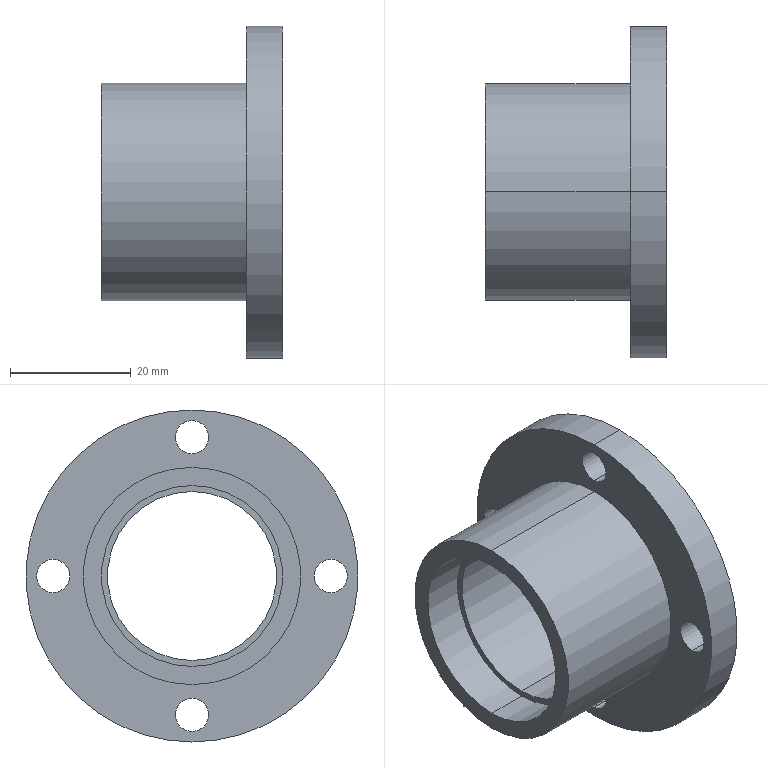Part | STEP file | MT-COMBO-119-S047 | 1 solid | 23 faces | box 30 x 55 x 55 mm | volume 18366 mm3 | cylinder 18 | plane 5 | commonest cylinder face diameters 5.5 x8 30 x4 28 x2 36 x2 55 x2
STEP:
#1=CARTESIAN_POINT('',(-6.,0.,-20.25));
#2=VERTEX_POINT('',#1);
#3=CARTESIAN_POINT('',(-6.,0.,-25.75));
#4=VERTEX_POINT('',#3);
#5=CARTESIAN_POINT('',(-6.,0.,-23.));
#6=DIRECTION('',(1.,0.,0.));
#7=DIRECTION('',(0.,0.,-1.));
#8=AXIS2_PLACEMENT_3D('',#5,#6,#7);
#9=CIRCLE('',#8,2.75);
#10=EDGE_CURVE('',#2,#4,#9,.T.);
#11=ORIENTED_EDGE('',*,*,#10,.F.);
#12=CARTESIAN_POINT('',(0.,0.,-20.25));
#13=VERTEX_POINT('',#12);
#14=CARTESIAN_POINT('',(0.,0.,-20.25));
#15=DIRECTION('',(1.,0.,0.));
#16=VECTOR('',#15,1000.);
#17=LINE('',#14,#16);
#18=EDGE_CURVE('',#2,#13,#17,.T.);
#19=ORIENTED_EDGE('',*,*,#18,.T.);
#20=CARTESIAN_POINT('',(0.,0.,-25.75));
#21=VERTEX_POINT('',#20);
#22=CARTESIAN_POINT('',(0.,0.,-23.));
#23=DIRECTION('',(1.,0.,0.));
#24=DIRECTION('',(0.,0.,-1.));
#25=AXIS2_PLACEMENT_3D('',#22,#23,#24);
#26=CIRCLE('',#25,2.75);
#27=EDGE_CURVE('',#13,#21,#26,.T.);
#28=ORIENTED_EDGE('',*,*,#27,.T.);
#29=CARTESIAN_POINT('',(0.,0.,-25.75));
#30=DIRECTION('',(1.,0.,0.));
#31=VECTOR('',#30,1000.);
#32=LINE('',#29,#31);
#33=EDGE_CURVE('',#4,#21,#32,.T.);
#34=ORIENTED_EDGE('',*,*,#33,.F.);
#35=EDGE_LOOP('',(#11,#19,#28,#34));
#36=FACE_OUTER_BOUND('',#35,.T.);
#37=CARTESIAN_POINT('',(0.,0.,-23.));
#38=DIRECTION('',(1.,0.,0.));
#39=DIRECTION('',(0.,0.,-1.));
#40=AXIS2_PLACEMENT_3D('',#37,#38,#39);
#41=CYLINDRICAL_SURFACE('',#40,2.75);
#42=ADVANCED_FACE('',(#36),#41,.F.);
#43=CARTESIAN_POINT('',(-6.,-23.,2.75));
#44=VERTEX_POINT('',#43);
#45=CARTESIAN_POINT('',(-6.,-23.,-2.75));
#46=VERTEX_POINT('',#45);
#47=CARTESIAN_POINT('',(-6.,-23.,0.));
#48=DIRECTION('',(1.,0.,0.));
#49=DIRECTION('',(0.,0.,-1.));
#50=AXIS2_PLACEMENT_3D('',#47,#48,#49);
#51=CIRCLE('',#50,2.75);
#52=EDGE_CURVE('',#44,#46,#51,.T.);
#53=ORIENTED_EDGE('',*,*,#52,.F.);
#54=CARTESIAN_POINT('',(0.,-23.,2.75));
#55=VERTEX_POINT('',#54);
#56=CARTESIAN_POINT('',(0.,-23.,2.75));
#57=DIRECTION('',(1.,0.,0.));
#58=VECTOR('',#57,1000.);
#59=LINE('',#56,#58);
#60=EDGE_CURVE('',#44,#55,#59,.T.);
#61=ORIENTED_EDGE('',*,*,#60,.T.);
#62=CARTESIAN_POINT('',(0.,-23.,-2.75));
#63=VERTEX_POINT('',#62);
#64=CARTESIAN_POINT('',(0.,-23.,0.));
#65=DIRECTION('',(1.,0.,0.));
#66=DIRECTION('',(0.,0.,-1.));
#67=AXIS2_PLACEMENT_3D('',#64,#65,#66);
#68=CIRCLE('',#67,2.75);
#69=EDGE_CURVE('',#55,#63,#68,.T.);
#70=ORIENTED_EDGE('',*,*,#69,.T.);
#71=CARTESIAN_POINT('',(0.,-23.,-2.75));
#72=DIRECTION('',(1.,0.,0.));
#73=VECTOR('',#72,1000.);
#74=LINE('',#71,#73);
#75=EDGE_CURVE('',#46,#63,#74,.T.);
#76=ORIENTED_EDGE('',*,*,#75,.F.);
#77=EDGE_LOOP('',(#53,#61,#70,#76));
#78=FACE_OUTER_BOUND('',#77,.T.);
#79=CARTESIAN_POINT('',(0.,-23.,0.));
#80=DIRECTION('',(1.,0.,0.));
#81=DIRECTION('',(0.,0.,-1.));
#82=AXIS2_PLACEMENT_3D('',#79,#80,#81);
#83=CYLINDRICAL_SURFACE('',#82,2.75);
#84=ADVANCED_FACE('',(#78),#83,.F.);
#85=CARTESIAN_POINT('',(-6.,0.,25.75));
#86=VERTEX_POINT('',#85);
#87=CARTESIAN_POINT('',(-6.,0.,20.25));
#88=VERTEX_POINT('',#87);
#89=CARTESIAN_POINT('',(-6.,0.,23.));
#90=DIRECTION('',(1.,0.,0.));
#91=DIRECTION('',(0.,0.,-1.));
#92=AXIS2_PLACEMENT_3D('',#89,#90,#91);
#93=CIRCLE('',#92,2.75);
#94=EDGE_CURVE('',#86,#88,#93,.T.);
#95=ORIENTED_EDGE('',*,*,#94,.F.);
#96=CARTESIAN_POINT('',(0.,0.,25.75));
#97=VERTEX_POINT('',#96);
#98=CARTESIAN_POINT('',(0.,0.,25.75));
#99=DIRECTION('',(1.,0.,0.));
#100=VECTOR('',#99,1000.);
#101=LINE('',#98,#100);
#102=EDGE_CURVE('',#86,#97,#101,.T.);
#103=ORIENTED_EDGE('',*,*,#102,.T.);
#104=CARTESIAN_POINT('',(0.,0.,20.25));
#105=VERTEX_POINT('',#104);
#106=CARTESIAN_POINT('',(0.,0.,23.));
#107=DIRECTION('',(1.,0.,0.));
#108=DIRECTION('',(0.,0.,-1.));
#109=AXIS2_PLACEMENT_3D('',#106,#107,#108);
#110=CIRCLE('',#109,2.75);
#111=EDGE_CURVE('',#97,#105,#110,.T.);
#112=ORIENTED_EDGE('',*,*,#111,.T.);
#113=CARTESIAN_POINT('',(0.,0.,20.25));
#114=DIRECTION('',(1.,0.,0.));
#115=VECTOR('',#114,1000.);
#116=LINE('',#113,#115);
#117=EDGE_CURVE('',#88,#105,#116,.T.);
#118=ORIENTED_EDGE('',*,*,#117,.F.);
#119=EDGE_LOOP('',(#95,#103,#112,#118));
#120=FACE_OUTER_BOUND('',#119,.T.);
#121=CARTESIAN_POINT('',(0.,0.,23.));
#122=DIRECTION('',(1.,0.,0.));
#123=DIRECTION('',(0.,0.,-1.));
#124=AXIS2_PLACEMENT_3D('',#121,#122,#123);
#125=CYLINDRICAL_SURFACE('',#124,2.75);
#126=ADVANCED_FACE('',(#120),#125,.F.);
#127=CARTESIAN_POINT('',(-6.,23.,2.75));
#128=VERTEX_POINT('',#127);
#129=CARTESIAN_POINT('',(-6.,23.,-2.75));
#130=VERTEX_POINT('',#129);
#131=CARTESIAN_POINT('',(-6.,23.,0.));
#132=DIRECTION('',(1.,0.,0.));
#133=DIRECTION('',(0.,0.,-1.));
#134=AXIS2_PLACEMENT_3D('',#131,#132,#133);
#135=CIRCLE('',#134,2.75);
#136=EDGE_CURVE('',#128,#130,#135,.T.);
#137=ORIENTED_EDGE('',*,*,#136,.F.);
#138=CARTESIAN_POINT('',(0.,23.,2.75));
#139=VERTEX_POINT('',#138);
#140=CARTESIAN_POINT('',(0.,23.,2.75));
#141=DIRECTION('',(1.,0.,0.));
#142=VECTOR('',#141,1000.);
#143=LINE('',#140,#142);
#144=EDGE_CURVE('',#128,#139,#143,.T.);
#145=ORIENTED_EDGE('',*,*,#144,.T.);
#146=CARTESIAN_POINT('',(0.,23.,-2.75));
#147=VERTEX_POINT('',#146);
#148=CARTESIAN_POINT('',(0.,23.,0.));
#149=DIRECTION('',(1.,0.,0.));
#150=DIRECTION('',(0.,0.,-1.));
#151=AXIS2_PLACEMENT_3D('',#148,#149,#150);
#152=CIRCLE('',#151,2.75);
#153=EDGE_CURVE('',#139,#147,#152,.T.);
#154=ORIENTED_EDGE('',*,*,#153,.T.);
#155=CARTESIAN_POINT('',(0.,23.,-2.75));
#156=DIRECTION('',(1.,0.,0.));
#157=VECTOR('',#156,1000.);
#158=LINE('',#155,#157);
#159=EDGE_CURVE('',#130,#147,#158,.T.);
#160=ORIENTED_EDGE('',*,*,#159,.F.);
#161=EDGE_LOOP('',(#137,#145,#154,#160));
#162=FACE_OUTER_BOUND('',#161,.T.);
#163=CARTESIAN_POINT('',(0.,23.,0.));
#164=DIRECTION('',(1.,0.,0.));
#165=DIRECTION('',(0.,0.,-1.));
#166=AXIS2_PLACEMENT_3D('',#163,#164,#165);
#167=CYLINDRICAL_SURFACE('',#166,2.75);
#168=ADVANCED_FACE('',(#162),#167,.F.);
#169=CARTESIAN_POINT('',(-7.,0.,-14.));
#170=VERTEX_POINT('',#169);
#171=CARTESIAN_POINT('',(-7.,0.,14.));
#172=VERTEX_POINT('',#171);
#173=CARTESIAN_POINT('',(-7.,0.,0.));
#174=DIRECTION('',(-1.,0.,0.));
#175=DIRECTION('',(0.,0.,1.));
#176=AXIS2_PLACEMENT_3D('',#173,#174,#175);
#177=CIRCLE('',#176,14.);
#178=EDGE_CURVE('',#170,#172,#177,.T.);
#179=ORIENTED_EDGE('',*,*,#178,.F.);
#180=CARTESIAN_POINT('',(-23.,0.,-14.));
#181=VERTEX_POINT('',#180);
#182=CARTESIAN_POINT('',(0.,0.,-14.));
#183=DIRECTION('',(-1.,0.,0.));
#184=VECTOR('',#183,1000.);
#185=LINE('',#182,#184);
#186=EDGE_CURVE('',#170,#181,#185,.T.);
#187=ORIENTED_EDGE('',*,*,#186,.T.);
#188=CARTESIAN_POINT('',(-23.,0.,14.));
#189=VERTEX_POINT('',#188);
#190=CARTESIAN_POINT('',(-23.,0.,0.));
#191=DIRECTION('',(-1.,0.,0.));
#192=DIRECTION('',(0.,0.,1.));
#193=AXIS2_PLACEMENT_3D('',#190,#191,#192);
#194=CIRCLE('',#193,14.);
#195=EDGE_CURVE('',#181,#189,#194,.T.);
#196=ORIENTED_EDGE('',*,*,#195,.T.);
#197=CARTESIAN_POINT('',(0.,0.,14.));
#198=DIRECTION('',(-1.,0.,0.));
#199=VECTOR('',#198,1000.);
#200=LINE('',#197,#199);
#201=EDGE_CURVE('',#172,#189,#200,.T.);
#202=ORIENTED_EDGE('',*,*,#201,.F.);
#203=EDGE_LOOP('',(#179,#187,#196,#202));
#204=FACE_OUTER_BOUND('',#203,.T.);
#205=CARTESIAN_POINT('',(0.,0.,0.));
#206=DIRECTION('',(-1.,0.,0.));
#207=DIRECTION('',(0.,0.,1.));
#208=AXIS2_PLACEMENT_3D('',#205,#206,#207);
#209=CYLINDRICAL_SURFACE('',#208,14.);
#210=ADVANCED_FACE('',(#204),#209,.F.);
#211=CARTESIAN_POINT('',(-23.,0.,-15.));
#212=VERTEX_POINT('',#211);
#213=CARTESIAN_POINT('',(-23.,0.,15.));
#214=VERTEX_POINT('',#213);
#215=CARTESIAN_POINT('',(-23.,0.,0.));
#216=DIRECTION('',(-1.,0.,0.));
#217=DIRECTION('',(0.,0.,1.));
#218=AXIS2_PLACEMENT_3D('',#215,#216,#217);
#219=CIRCLE('',#218,15.);
#220=EDGE_CURVE('',#212,#214,#219,.T.);
#221=ORIENTED_EDGE('',*,*,#220,.F.);
#222=CARTESIAN_POINT('',(-30.,0.,-15.));
#223=VERTEX_POINT('',#222);
#224=CARTESIAN_POINT('',(0.,0.,-15.));
#225=DIRECTION('',(-1.,0.,0.));
#226=VECTOR('',#225,1000.);
#227=LINE('',#224,#226);
#228=EDGE_CURVE('',#212,#223,#227,.T.);
#229=ORIENTED_EDGE('',*,*,#228,.T.);
#230=CARTESIAN_POINT('',(-30.,0.,15.));
#231=VERTEX_POINT('',#230);
#232=CARTESIAN_POINT('',(-30.,0.,0.));
#233=DIRECTION('',(-1.,0.,0.));
#234=DIRECTION('',(0.,0.,1.));
#235=AXIS2_PLACEMENT_3D('',#232,#233,#234);
#236=CIRCLE('',#235,15.);
#237=EDGE_CURVE('',#223,#231,#236,.T.);
#238=ORIENTED_EDGE('',*,*,#237,.T.);
#239=CARTESIAN_POINT('',(0.,0.,15.));
#240=DIRECTION('',(-1.,0.,0.));
#241=VECTOR('',#240,1000.);
#242=LINE('',#239,#241);
#243=EDGE_CURVE('',#214,#231,#242,.T.);
#244=ORIENTED_EDGE('',*,*,#243,.F.);
#245=EDGE_LOOP('',(#221,#229,#238,#244));
#246=FACE_OUTER_BOUND('',#245,.T.);
#247=CARTESIAN_POINT('',(0.,0.,0.));
#248=DIRECTION('',(-1.,0.,0.));
#249=DIRECTION('',(0.,0.,1.));
#250=AXIS2_PLACEMENT_3D('',#247,#248,#249);
#251=CYLINDRICAL_SURFACE('',#250,15.);
#252=ADVANCED_FACE('',(#246),#251,.F.);
#253=CARTESIAN_POINT('',(-6.,0.,18.));
#254=VERTEX_POINT('',#253);
#255=CARTESIAN_POINT('',(-6.,0.,-18.));
#256=VERTEX_POINT('',#255);
#257=CARTESIAN_POINT('',(-6.,0.,0.));
#258=DIRECTION('',(-1.,0.,0.));
#259=DIRECTION('',(0.,0.,1.));
#260=AXIS2_PLACEMENT_3D('',#257,#258,#259);
#261=CIRCLE('',#260,18.);
#262=EDGE_CURVE('',#254,#256,#261,.T.);
#263=ORIENTED_EDGE('',*,*,#262,.T.);
#264=CARTESIAN_POINT('',(-30.,0.,-18.));
#265=VERTEX_POINT('',#264);
#266=CARTESIAN_POINT('',(0.,0.,-18.));
#267=DIRECTION('',(-1.,0.,0.));
#268=VECTOR('',#267,1000.);
#269=LINE('',#266,#268);
#270=EDGE_CURVE('',#256,#265,#269,.T.);
#271=ORIENTED_EDGE('',*,*,#270,.T.);
#272=CARTESIAN_POINT('',(-30.,0.,18.));
#273=VERTEX_POINT('',#272);
#274=CARTESIAN_POINT('',(-30.,0.,0.));
#275=DIRECTION('',(-1.,0.,0.));
#276=DIRECTION('',(0.,0.,1.));
#277=AXIS2_PLACEMENT_3D('',#274,#275,#276);
#278=CIRCLE('',#277,18.);
#279=EDGE_CURVE('',#273,#265,#278,.T.);
#280=ORIENTED_EDGE('',*,*,#279,.F.);
#281=CARTESIAN_POINT('',(0.,0.,18.));
#282=DIRECTION('',(-1.,0.,0.));
#283=VECTOR('',#282,1000.);
#284=LINE('',#281,#283);
#285=EDGE_CURVE('',#254,#273,#284,.T.);
#286=ORIENTED_EDGE('',*,*,#285,.F.);
#287=EDGE_LOOP('',(#263,#271,#280,#286));
#288=FACE_OUTER_BOUND('',#287,.T.);
#289=CARTESIAN_POINT('',(0.,0.,0.));
#290=DIRECTION('',(-1.,0.,0.));
#291=DIRECTION('',(0.,0.,1.));
#292=AXIS2_PLACEMENT_3D('',#289,#290,#291);
#293=CYLINDRICAL_SURFACE('',#292,18.);
#294=ADVANCED_FACE('',(#288),#293,.T.);
#295=CARTESIAN_POINT('',(0.,0.,27.5));
#296=VERTEX_POINT('',#295);
#297=CARTESIAN_POINT('',(0.,0.,-27.5));
#298=VERTEX_POINT('',#297);
#299=CARTESIAN_POINT('',(0.,0.,0.));
#300=DIRECTION('',(-1.,0.,0.));
#301=DIRECTION('',(0.,0.,1.));
#302=AXIS2_PLACEMENT_3D('',#299,#300,#301);
#303=CIRCLE('',#302,27.5);
#304=EDGE_CURVE('',#296,#298,#303,.T.);
#305=ORIENTED_EDGE('',*,*,#304,.T.);
#306=CARTESIAN_POINT('',(-6.,0.,-27.5));
#307=VERTEX_POINT('',#306);
#308=CARTESIAN_POINT('',(0.,0.,-27.5));
#309=DIRECTION('',(-1.,0.,0.));
#310=VECTOR('',#309,1000.);
#311=LINE('',#308,#310);
#312=EDGE_CURVE('',#298,#307,#311,.T.);
#313=ORIENTED_EDGE('',*,*,#312,.T.);
#314=CARTESIAN_POINT('',(-6.,0.,27.5));
#315=VERTEX_POINT('',#314);
#316=CARTESIAN_POINT('',(-6.,0.,0.));
#317=DIRECTION('',(-1.,0.,0.));
#318=DIRECTION('',(0.,0.,1.));
#319=AXIS2_PLACEMENT_3D('',#316,#317,#318);
#320=CIRCLE('',#319,27.5);
#321=EDGE_CURVE('',#315,#307,#320,.T.);
#322=ORIENTED_EDGE('',*,*,#321,.F.);
#323=CARTESIAN_POINT('',(0.,0.,27.5));
#324=DIRECTION('',(-1.,0.,0.));
#325=VECTOR('',#324,1000.);
#326=LINE('',#323,#325);
#327=EDGE_CURVE('',#296,#315,#326,.T.);
#328=ORIENTED_EDGE('',*,*,#327,.F.);
#329=EDGE_LOOP('',(#305,#313,#322,#328));
#330=FACE_OUTER_BOUND('',#329,.T.);
#331=CARTESIAN_POINT('',(0.,0.,0.));
#332=DIRECTION('',(-1.,0.,0.));
#333=DIRECTION('',(0.,0.,1.));
#334=AXIS2_PLACEMENT_3D('',#331,#332,#333);
#335=CYLINDRICAL_SURFACE('',#334,27.5);
#336=ADVANCED_FACE('',(#330),#335,.T.);
#337=CARTESIAN_POINT('',(0.,0.,-15.));
#338=VERTEX_POINT('',#337);
#339=CARTESIAN_POINT('',(0.,0.,15.));
#340=VERTEX_POINT('',#339);
#341=CARTESIAN_POINT('',(0.,0.,0.));
#342=DIRECTION('',(-1.,0.,0.));
#343=DIRECTION('',(0.,0.,1.));
#344=AXIS2_PLACEMENT_3D('',#341,#342,#343);
#345=CIRCLE('',#344,15.);
#346=EDGE_CURVE('',#338,#340,#345,.T.);
#347=ORIENTED_EDGE('',*,*,#346,.F.);
#348=CARTESIAN_POINT('',(-7.,0.,-15.));
#349=VERTEX_POINT('',#348);
#350=CARTESIAN_POINT('',(0.,0.,-15.));
#351=DIRECTION('',(-1.,0.,0.));
#352=VECTOR('',#351,1000.);
#353=LINE('',#350,#352);
#354=EDGE_CURVE('',#338,#349,#353,.T.);
#355=ORIENTED_EDGE('',*,*,#354,.T.);
#356=CARTESIAN_POINT('',(-7.,0.,15.));
#357=VERTEX_POINT('',#356);
#358=CARTESIAN_POINT('',(-7.,0.,0.));
#359=DIRECTION('',(-1.,0.,0.));
#360=DIRECTION('',(0.,0.,1.));
#361=AXIS2_PLACEMENT_3D('',#358,#359,#360);
#362=CIRCLE('',#361,15.);
#363=EDGE_CURVE('',#349,#357,#362,.T.);
#364=ORIENTED_EDGE('',*,*,#363,.T.);
#365=CARTESIAN_POINT('',(0.,0.,15.));
#366=DIRECTION('',(-1.,0.,0.));
#367=VECTOR('',#366,1000.);
#368=LINE('',#365,#367);
#369=EDGE_CURVE('',#340,#357,#368,.T.);
#370=ORIENTED_EDGE('',*,*,#369,.F.);
#371=EDGE_LOOP('',(#347,#355,#364,#370));
#372=FACE_OUTER_BOUND('',#371,.T.);
#373=CARTESIAN_POINT('',(0.,0.,0.));
#374=DIRECTION('',(-1.,0.,0.));
#375=DIRECTION('',(0.,0.,1.));
#376=AXIS2_PLACEMENT_3D('',#373,#374,#375);
#377=CYLINDRICAL_SURFACE('',#376,15.);
#378=ADVANCED_FACE('',(#372),#377,.F.);
#379=ORIENTED_EDGE('',*,*,#354,.F.);
#380=CARTESIAN_POINT('',(0.,0.,0.));
#381=DIRECTION('',(-1.,0.,0.));
#382=DIRECTION('',(0.,0.,1.));
#383=AXIS2_PLACEMENT_3D('',#380,#381,#382);
#384=CIRCLE('',#383,15.);
#385=EDGE_CURVE('',#340,#338,#384,.T.);
#386=ORIENTED_EDGE('',*,*,#385,.F.);
#387=ORIENTED_EDGE('',*,*,#369,.T.);
#388=CARTESIAN_POINT('',(-7.,0.,0.));
#389=DIRECTION('',(-1.,0.,0.));
#390=DIRECTION('',(0.,0.,1.));
#391=AXIS2_PLACEMENT_3D('',#388,#389,#390);
#392=CIRCLE('',#391,15.);
#393=EDGE_CURVE('',#357,#349,#392,.T.);
#394=ORIENTED_EDGE('',*,*,#393,.T.);
#395=EDGE_LOOP('',(#379,#386,#387,#394));
#396=FACE_OUTER_BOUND('',#395,.T.);
#397=CARTESIAN_POINT('',(0.,0.,0.));
#398=DIRECTION('',(-1.,0.,0.));
#399=DIRECTION('',(0.,0.,1.));
#400=AXIS2_PLACEMENT_3D('',#397,#398,#399);
#401=CYLINDRICAL_SURFACE('',#400,15.);
#402=ADVANCED_FACE('',(#396),#401,.F.);
#403=CARTESIAN_POINT('',(0.,0.,-23.));
#404=DIRECTION('',(1.,0.,0.));
#405=DIRECTION('',(0.,0.,-1.));
#406=AXIS2_PLACEMENT_3D('',#403,#404,#405);
#407=CIRCLE('',#406,2.75);
#408=EDGE_CURVE('',#21,#13,#407,.T.);
#409=ORIENTED_EDGE('',*,*,#408,.F.);
#410=ORIENTED_EDGE('',*,*,#27,.F.);
#411=EDGE_LOOP('',(#409,#410));
#412=FACE_BOUND('',#411,.T.);
#413=CARTESIAN_POINT('',(0.,-23.,0.));
#414=DIRECTION('',(1.,0.,0.));
#415=DIRECTION('',(0.,0.,-1.));
#416=AXIS2_PLACEMENT_3D('',#413,#414,#415);
#417=CIRCLE('',#416,2.75);
#418=EDGE_CURVE('',#63,#55,#417,.T.);
#419=ORIENTED_EDGE('',*,*,#418,.F.);
#420=ORIENTED_EDGE('',*,*,#69,.F.);
#421=EDGE_LOOP('',(#419,#420));
#422=FACE_BOUND('',#421,.T.);
#423=CARTESIAN_POINT('',(0.,0.,23.));
#424=DIRECTION('',(1.,0.,0.));
#425=DIRECTION('',(0.,0.,-1.));
#426=AXIS2_PLACEMENT_3D('',#423,#424,#425);
#427=CIRCLE('',#426,2.75);
#428=EDGE_CURVE('',#105,#97,#427,.T.);
#429=ORIENTED_EDGE('',*,*,#428,.F.);
#430=ORIENTED_EDGE('',*,*,#111,.F.);
#431=EDGE_LOOP('',(#429,#430));
#432=FACE_BOUND('',#431,.T.);
#433=CARTESIAN_POINT('',(0.,23.,0.));
#434=DIRECTION('',(1.,0.,0.));
#435=DIRECTION('',(0.,0.,-1.));
#436=AXIS2_PLACEMENT_3D('',#433,#434,#435);
#437=CIRCLE('',#436,2.75);
#438=EDGE_CURVE('',#147,#139,#437,.T.);
#439=ORIENTED_EDGE('',*,*,#438,.F.);
#440=ORIENTED_EDGE('',*,*,#153,.F.);
#441=EDGE_LOOP('',(#439,#440));
#442=FACE_BOUND('',#441,.T.);
#443=ORIENTED_EDGE('',*,*,#304,.F.);
#444=CARTESIAN_POINT('',(0.,0.,0.));
#445=DIRECTION('',(-1.,0.,0.));
#446=DIRECTION('',(0.,0.,1.));
#447=AXIS2_PLACEMENT_3D('',#444,#445,#446);
#448=CIRCLE('',#447,27.5);
#449=EDGE_CURVE('',#298,#296,#448,.T.);
#450=ORIENTED_EDGE('',*,*,#449,.F.);
#451=EDGE_LOOP('',(#443,#450));
#452=FACE_OUTER_BOUND('',#451,.T.);
#453=ORIENTED_EDGE('',*,*,#385,.T.);
#454=ORIENTED_EDGE('',*,*,#346,.T.);
#455=EDGE_LOOP('',(#453,#454));
#456=FACE_BOUND('',#455,.T.);
#457=CARTESIAN_POINT('',(0.,15.,0.));
#458=DIRECTION('',(-1.,0.,0.));
#459=DIRECTION('',(0.,0.,1.));
#460=AXIS2_PLACEMENT_3D('',#457,#458,#459);
#461=PLANE('',#460);
#462=ADVANCED_FACE('',(#412,#422,#432,#442,#452,#456),#461,.F.);
#463=ORIENTED_EDGE('',*,*,#312,.F.);
#464=ORIENTED_EDGE('',*,*,#449,.T.);
#465=ORIENTED_EDGE('',*,*,#327,.T.);
#466=CARTESIAN_POINT('',(-6.,0.,0.));
#467=DIRECTION('',(-1.,0.,0.));
#468=DIRECTION('',(0.,0.,1.));
#469=AXIS2_PLACEMENT_3D('',#466,#467,#468);
#470=CIRCLE('',#469,27.5);
#471=EDGE_CURVE('',#307,#315,#470,.T.);
#472=ORIENTED_EDGE('',*,*,#471,.F.);
#473=EDGE_LOOP('',(#463,#464,#465,#472));
#474=FACE_OUTER_BOUND('',#473,.T.);
#475=CARTESIAN_POINT('',(0.,0.,0.));
#476=DIRECTION('',(-1.,0.,0.));
#477=DIRECTION('',(0.,0.,1.));
#478=AXIS2_PLACEMENT_3D('',#475,#476,#477);
#479=CYLINDRICAL_SURFACE('',#478,27.5);
#480=ADVANCED_FACE('',(#474),#479,.T.);
#481=CARTESIAN_POINT('',(-6.,0.,-23.));
#482=DIRECTION('',(1.,0.,0.));
#483=DIRECTION('',(0.,0.,-1.));
#484=AXIS2_PLACEMENT_3D('',#481,#482,#483);
#485=CIRCLE('',#484,2.75);
#486=EDGE_CURVE('',#4,#2,#485,.T.);
#487=ORIENTED_EDGE('',*,*,#486,.T.);
#488=ORIENTED_EDGE('',*,*,#10,.T.);
#489=EDGE_LOOP('',(#487,#488));
#490=FACE_BOUND('',#489,.T.);
#491=CARTESIAN_POINT('',(-6.,-23.,0.));
#492=DIRECTION('',(1.,0.,0.));
#493=DIRECTION('',(0.,0.,-1.));
#494=AXIS2_PLACEMENT_3D('',#491,#492,#493);
#495=CIRCLE('',#494,2.75);
#496=EDGE_CURVE('',#46,#44,#495,.T.);
#497=ORIENTED_EDGE('',*,*,#496,.T.);
#498=ORIENTED_EDGE('',*,*,#52,.T.);
#499=EDGE_LOOP('',(#497,#498));
#500=FACE_BOUND('',#499,.T.);
#501=CARTESIAN_POINT('',(-6.,0.,23.));
#502=DIRECTION('',(1.,0.,0.));
#503=DIRECTION('',(0.,0.,-1.));
#504=AXIS2_PLACEMENT_3D('',#501,#502,#503);
#505=CIRCLE('',#504,2.75);
#506=EDGE_CURVE('',#88,#86,#505,.T.);
#507=ORIENTED_EDGE('',*,*,#506,.T.);
#508=ORIENTED_EDGE('',*,*,#94,.T.);
#509=EDGE_LOOP('',(#507,#508));
#510=FACE_BOUND('',#509,.T.);
#511=CARTESIAN_POINT('',(-6.,23.,0.));
#512=DIRECTION('',(1.,0.,0.));
#513=DIRECTION('',(0.,0.,-1.));
#514=AXIS2_PLACEMENT_3D('',#511,#512,#513);
#515=CIRCLE('',#514,2.75);
#516=EDGE_CURVE('',#130,#128,#515,.T.);
#517=ORIENTED_EDGE('',*,*,#516,.T.);
#518=ORIENTED_EDGE('',*,*,#136,.T.);
#519=EDGE_LOOP('',(#517,#518));
#520=FACE_BOUND('',#519,.T.);
#521=ORIENTED_EDGE('',*,*,#262,.F.);
#522=CARTESIAN_POINT('',(-6.,0.,0.));
#523=DIRECTION('',(-1.,0.,0.));
#524=DIRECTION('',(0.,0.,1.));
#525=AXIS2_PLACEMENT_3D('',#522,#523,#524);
#526=CIRCLE('',#525,18.);
#527=EDGE_CURVE('',#256,#254,#526,.T.);
#528=ORIENTED_EDGE('',*,*,#527,.F.);
#529=EDGE_LOOP('',(#521,#528));
#530=FACE_BOUND('',#529,.T.);
#531=ORIENTED_EDGE('',*,*,#321,.T.);
#532=ORIENTED_EDGE('',*,*,#471,.T.);
#533=EDGE_LOOP('',(#531,#532));
#534=FACE_OUTER_BOUND('',#533,.T.);
#535=CARTESIAN_POINT('',(-6.,27.5,0.));
#536=DIRECTION('',(1.,0.,0.));
#537=DIRECTION('',(0.,0.,-1.));
#538=AXIS2_PLACEMENT_3D('',#535,#536,#537);
#539=PLANE('',#538);
#540=ADVANCED_FACE('',(#490,#500,#510,#520,#530,#534),#539,.F.);
#541=ORIENTED_EDGE('',*,*,#270,.F.);
#542=ORIENTED_EDGE('',*,*,#527,.T.);
#543=ORIENTED_EDGE('',*,*,#285,.T.);
#544=CARTESIAN_POINT('',(-30.,0.,0.));
#545=DIRECTION('',(-1.,0.,0.));
#546=DIRECTION('',(0.,0.,1.));
#547=AXIS2_PLACEMENT_3D('',#544,#545,#546);
#548=CIRCLE('',#547,18.);
#549=EDGE_CURVE('',#265,#273,#548,.T.);
#550=ORIENTED_EDGE('',*,*,#549,.F.);
#551=EDGE_LOOP('',(#541,#542,#543,#550));
#552=FACE_OUTER_BOUND('',#551,.T.);
#553=CARTESIAN_POINT('',(0.,0.,0.));
#554=DIRECTION('',(-1.,0.,0.));
#555=DIRECTION('',(0.,0.,1.));
#556=AXIS2_PLACEMENT_3D('',#553,#554,#555);
#557=CYLINDRICAL_SURFACE('',#556,18.);
#558=ADVANCED_FACE('',(#552),#557,.T.);
#559=CARTESIAN_POINT('',(-30.,0.,0.));
#560=DIRECTION('',(-1.,0.,0.));
#561=DIRECTION('',(0.,0.,1.));
#562=AXIS2_PLACEMENT_3D('',#559,#560,#561);
#563=CIRCLE('',#562,15.);
#564=EDGE_CURVE('',#231,#223,#563,.T.);
#565=ORIENTED_EDGE('',*,*,#564,.F.);
#566=ORIENTED_EDGE('',*,*,#237,.F.);
#567=EDGE_LOOP('',(#565,#566));
#568=FACE_BOUND('',#567,.T.);
#569=ORIENTED_EDGE('',*,*,#279,.T.);
#570=ORIENTED_EDGE('',*,*,#549,.T.);
#571=EDGE_LOOP('',(#569,#570));
#572=FACE_OUTER_BOUND('',#571,.T.);
#573=CARTESIAN_POINT('',(-30.,18.,0.));
#574=DIRECTION('',(1.,0.,0.));
#575=DIRECTION('',(0.,0.,-1.));
#576=AXIS2_PLACEMENT_3D('',#573,#574,#575);
#577=PLANE('',#576);
#578=ADVANCED_FACE('',(#568,#572),#577,.F.);
#579=ORIENTED_EDGE('',*,*,#228,.F.);
#580=CARTESIAN_POINT('',(-23.,0.,0.));
#581=DIRECTION('',(-1.,0.,0.));
#582=DIRECTION('',(0.,0.,1.));
#583=AXIS2_PLACEMENT_3D('',#580,#581,#582);
#584=CIRCLE('',#583,15.);
#585=EDGE_CURVE('',#214,#212,#584,.T.);
#586=ORIENTED_EDGE('',*,*,#585,.F.);
#587=ORIENTED_EDGE('',*,*,#243,.T.);
#588=ORIENTED_EDGE('',*,*,#564,.T.);
#589=EDGE_LOOP('',(#579,#586,#587,#588));
#590=FACE_OUTER_BOUND('',#589,.T.);
#591=CARTESIAN_POINT('',(0.,0.,0.));
#592=DIRECTION('',(-1.,0.,0.));
#593=DIRECTION('',(0.,0.,1.));
#594=AXIS2_PLACEMENT_3D('',#591,#592,#593);
#595=CYLINDRICAL_SURFACE('',#594,15.);
#596=ADVANCED_FACE('',(#590),#595,.F.);
#597=CARTESIAN_POINT('',(-23.,0.,0.));
#598=DIRECTION('',(-1.,0.,0.));
#599=DIRECTION('',(0.,0.,1.));
#600=AXIS2_PLACEMENT_3D('',#597,#598,#599);
#601=CIRCLE('',#600,14.);
#602=EDGE_CURVE('',#189,#181,#601,.T.);
#603=ORIENTED_EDGE('',*,*,#602,.F.);
#604=ORIENTED_EDGE('',*,*,#195,.F.);
#605=EDGE_LOOP('',(#603,#604));
#606=FACE_BOUND('',#605,.T.);
#607=ORIENTED_EDGE('',*,*,#585,.T.);
#608=ORIENTED_EDGE('',*,*,#220,.T.);
#609=EDGE_LOOP('',(#607,#608));
#610=FACE_OUTER_BOUND('',#609,.T.);
#611=CARTESIAN_POINT('',(-23.,15.,0.));
#612=DIRECTION('',(1.,0.,0.));
#613=DIRECTION('',(0.,0.,-1.));
#614=AXIS2_PLACEMENT_3D('',#611,#612,#613);
#615=PLANE('',#614);
#616=ADVANCED_FACE('',(#606,#610),#615,.F.);
#617=ORIENTED_EDGE('',*,*,#186,.F.);
#618=CARTESIAN_POINT('',(-7.,0.,0.));
#619=DIRECTION('',(-1.,0.,0.));
#620=DIRECTION('',(0.,0.,1.));
#621=AXIS2_PLACEMENT_3D('',#618,#619,#620);
#622=CIRCLE('',#621,14.);
#623=EDGE_CURVE('',#172,#170,#622,.T.);
#624=ORIENTED_EDGE('',*,*,#623,.F.);
#625=ORIENTED_EDGE('',*,*,#201,.T.);
#626=ORIENTED_EDGE('',*,*,#602,.T.);
#627=EDGE_LOOP('',(#617,#624,#625,#626));
#628=FACE_OUTER_BOUND('',#627,.T.);
#629=CARTESIAN_POINT('',(0.,0.,0.));
#630=DIRECTION('',(-1.,0.,0.));
#631=DIRECTION('',(0.,0.,1.));
#632=AXIS2_PLACEMENT_3D('',#629,#630,#631);
#633=CYLINDRICAL_SURFACE('',#632,14.);
#634=ADVANCED_FACE('',(#628),#633,.F.);
#635=ORIENTED_EDGE('',*,*,#393,.F.);
#636=ORIENTED_EDGE('',*,*,#363,.F.);
#637=EDGE_LOOP('',(#635,#636));
#638=FACE_OUTER_BOUND('',#637,.T.);
#639=ORIENTED_EDGE('',*,*,#623,.T.);
#640=ORIENTED_EDGE('',*,*,#178,.T.);
#641=EDGE_LOOP('',(#639,#640));
#642=FACE_BOUND('',#641,.T.);
#643=CARTESIAN_POINT('',(-7.,14.,0.));
#644=DIRECTION('',(-1.,0.,0.));
#645=DIRECTION('',(0.,0.,1.));
#646=AXIS2_PLACEMENT_3D('',#643,#644,#645);
#647=PLANE('',#646);
#648=ADVANCED_FACE('',(#638,#642),#647,.F.);
#649=ORIENTED_EDGE('',*,*,#144,.F.);
#650=ORIENTED_EDGE('',*,*,#516,.F.);
#651=ORIENTED_EDGE('',*,*,#159,.T.);
#652=ORIENTED_EDGE('',*,*,#438,.T.);
#653=EDGE_LOOP('',(#649,#650,#651,#652));
#654=FACE_OUTER_BOUND('',#653,.T.);
#655=CARTESIAN_POINT('',(0.,23.,0.));
#656=DIRECTION('',(1.,0.,0.));
#657=DIRECTION('',(0.,0.,-1.));
#658=AXIS2_PLACEMENT_3D('',#655,#656,#657);
#659=CYLINDRICAL_SURFACE('',#658,2.75);
#660=ADVANCED_FACE('',(#654),#659,.F.);
#661=ORIENTED_EDGE('',*,*,#102,.F.);
#662=ORIENTED_EDGE('',*,*,#506,.F.);
#663=ORIENTED_EDGE('',*,*,#117,.T.);
#664=ORIENTED_EDGE('',*,*,#428,.T.);
#665=EDGE_LOOP('',(#661,#662,#663,#664));
#666=FACE_OUTER_BOUND('',#665,.T.);
#667=CARTESIAN_POINT('',(0.,0.,23.));
#668=DIRECTION('',(1.,0.,0.));
#669=DIRECTION('',(0.,0.,-1.));
#670=AXIS2_PLACEMENT_3D('',#667,#668,#669);
#671=CYLINDRICAL_SURFACE('',#670,2.75);
#672=ADVANCED_FACE('',(#666),#671,.F.);
#673=ORIENTED_EDGE('',*,*,#60,.F.);
#674=ORIENTED_EDGE('',*,*,#496,.F.);
#675=ORIENTED_EDGE('',*,*,#75,.T.);
#676=ORIENTED_EDGE('',*,*,#418,.T.);
#677=EDGE_LOOP('',(#673,#674,#675,#676));
#678=FACE_OUTER_BOUND('',#677,.T.);
#679=CARTESIAN_POINT('',(0.,-23.,0.));
#680=DIRECTION('',(1.,0.,0.));
#681=DIRECTION('',(0.,0.,-1.));
#682=AXIS2_PLACEMENT_3D('',#679,#680,#681);
#683=CYLINDRICAL_SURFACE('',#682,2.75);
#684=ADVANCED_FACE('',(#678),#683,.F.);
#685=ORIENTED_EDGE('',*,*,#18,.F.);
#686=ORIENTED_EDGE('',*,*,#486,.F.);
#687=ORIENTED_EDGE('',*,*,#33,.T.);
#688=ORIENTED_EDGE('',*,*,#408,.T.);
#689=EDGE_LOOP('',(#685,#686,#687,#688));
#690=FACE_OUTER_BOUND('',#689,.T.);
#691=CARTESIAN_POINT('',(0.,0.,-23.));
#692=DIRECTION('',(1.,0.,0.));
#693=DIRECTION('',(0.,0.,-1.));
#694=AXIS2_PLACEMENT_3D('',#691,#692,#693);
#695=CYLINDRICAL_SURFACE('',#694,2.75);
#696=ADVANCED_FACE('',(#690),#695,.F.);
#697=CLOSED_SHELL('',(#42,#84,#126,#168,#210,#252,#294,#336,#378,#402,#462,#480,#540,#558,#578,#596,#616,#634,#648,#660,#672,#684,#696));
#698=MANIFOLD_SOLID_BREP('',#697);
#699=CARTESIAN_POINT('',(0.,0.,0.));
#700=DIRECTION('',(0.,0.,1.));
#701=DIRECTION('',(1.,0.,0.));
#702=AXIS2_PLACEMENT_3D('',#699,#700,#701);
#703=(LENGTH_UNIT()NAMED_UNIT(*)SI_UNIT(.MILLI.,.METRE.));
#704=UNCERTAINTY_MEASURE_WITH_UNIT(LENGTH_MEASURE(0.00001),#703,'','');
#705=(NAMED_UNIT(*)PLANE_ANGLE_UNIT()SI_UNIT($,.RADIAN.));
#706=(NAMED_UNIT(*)SI_UNIT($,.STERADIAN.)SOLID_ANGLE_UNIT());
#707=(GEOMETRIC_REPRESENTATION_CONTEXT(3)GLOBAL_UNCERTAINTY_ASSIGNED_CONTEXT((#704))GLOBAL_UNIT_ASSIGNED_CONTEXT((#703,#705,#706))REPRESENTATION_CONTEXT('',''));
#708=ADVANCED_BREP_SHAPE_REPRESENTATION('',(#698,#702),#707);